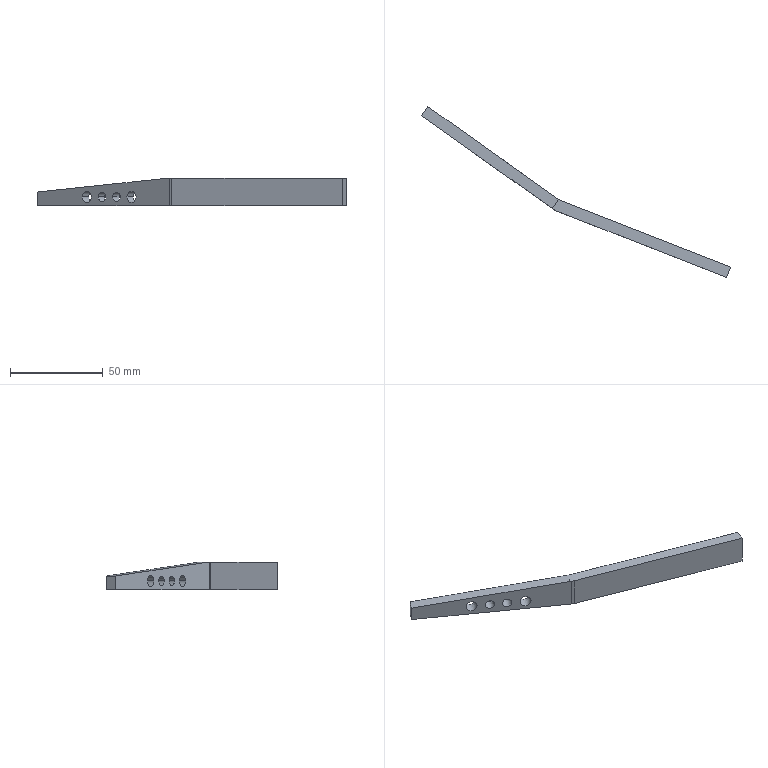Part | SolidWorks | features HoleWzd 2, Cut 1, Extrusion 1 | 1 solid | 19 faces | box 166.528 x 92.061 x 15 mm | volume 14282 mm3 | cylinder 10 | plane 9 | commonest cylinder face diameters 5 x4 6 x4 12 x2
STEP:
#1=CARTESIAN_POINT('',(-108.721,171.607,4.871));
#2=VERTEX_POINT('',#1);
#3=CARTESIAN_POINT('',(-112.797,174.503,4.871));
#4=VERTEX_POINT('',#3);
#5=CARTESIAN_POINT('',(-110.759,173.055,4.871));
#6=DIRECTION('',(0.5792,0.8152,0.));
#7=DIRECTION('',(-0.8152,0.5792,0.));
#8=AXIS2_PLACEMENT_3D('',#5,#6,#7);
#9=CIRCLE('',#8,2.5);
#10=EDGE_CURVE('',#2,#4,#9,.T.);
#11=ORIENTED_EDGE('',*,*,#10,.F.);
#12=CARTESIAN_POINT('',(-105.245,176.498,4.871));
#13=VERTEX_POINT('',#12);
#14=CARTESIAN_POINT('',(-105.245,176.498,4.871));
#15=DIRECTION('',(0.5792,0.8152,0.));
#16=VECTOR('',#15,1000.);
#17=LINE('',#14,#16);
#18=EDGE_CURVE('',#2,#13,#17,.T.);
#19=ORIENTED_EDGE('',*,*,#18,.T.);
#20=CARTESIAN_POINT('',(-109.321,179.394,4.871));
#21=VERTEX_POINT('',#20);
#22=CARTESIAN_POINT('',(-107.283,177.946,4.871));
#23=DIRECTION('',(0.5792,0.8152,0.));
#24=DIRECTION('',(-0.8152,0.5792,0.));
#25=AXIS2_PLACEMENT_3D('',#22,#23,#24);
#26=CIRCLE('',#25,2.5);
#27=EDGE_CURVE('',#13,#21,#26,.T.);
#28=ORIENTED_EDGE('',*,*,#27,.T.);
#29=CARTESIAN_POINT('',(-109.321,179.394,4.871));
#30=DIRECTION('',(0.5792,0.8152,0.));
#31=VECTOR('',#30,1000.);
#32=LINE('',#29,#31);
#33=EDGE_CURVE('',#4,#21,#32,.T.);
#34=ORIENTED_EDGE('',*,*,#33,.F.);
#35=EDGE_LOOP('',(#11,#19,#28,#34));
#36=FACE_OUTER_BOUND('',#35,.T.);
#37=CARTESIAN_POINT('',(-107.283,177.946,4.871));
#38=DIRECTION('',(0.5792,0.8152,0.));
#39=DIRECTION('',(-0.8152,0.5792,0.));
#40=AXIS2_PLACEMENT_3D('',#37,#38,#39);
#41=CYLINDRICAL_SURFACE('',#40,2.5);
#42=ADVANCED_FACE('',(#36),#41,.F.);
#43=CARTESIAN_POINT('',(-100.99,166.114,4.871));
#44=VERTEX_POINT('',#43);
#45=CARTESIAN_POINT('',(-105.066,169.01,4.871));
#46=VERTEX_POINT('',#45);
#47=CARTESIAN_POINT('',(-103.028,167.562,4.871));
#48=DIRECTION('',(0.5792,0.8152,0.));
#49=DIRECTION('',(-0.8152,0.5792,0.));
#50=AXIS2_PLACEMENT_3D('',#47,#48,#49);
#51=CIRCLE('',#50,2.5);
#52=EDGE_CURVE('',#44,#46,#51,.T.);
#53=ORIENTED_EDGE('',*,*,#52,.F.);
#54=CARTESIAN_POINT('',(-97.515,171.005,4.871));
#55=VERTEX_POINT('',#54);
#56=CARTESIAN_POINT('',(-97.515,171.005,4.871));
#57=DIRECTION('',(0.5792,0.8152,0.));
#58=VECTOR('',#57,1000.);
#59=LINE('',#56,#58);
#60=EDGE_CURVE('',#44,#55,#59,.T.);
#61=ORIENTED_EDGE('',*,*,#60,.T.);
#62=CARTESIAN_POINT('',(-101.591,173.901,4.871));
#63=VERTEX_POINT('',#62);
#64=CARTESIAN_POINT('',(-99.553,172.453,4.871));
#65=DIRECTION('',(0.5792,0.8152,0.));
#66=DIRECTION('',(-0.8152,0.5792,0.));
#67=AXIS2_PLACEMENT_3D('',#64,#65,#66);
#68=CIRCLE('',#67,2.5);
#69=EDGE_CURVE('',#55,#63,#68,.T.);
#70=ORIENTED_EDGE('',*,*,#69,.T.);
#71=CARTESIAN_POINT('',(-101.591,173.901,4.871));
#72=DIRECTION('',(0.5792,0.8152,0.));
#73=VECTOR('',#72,1000.);
#74=LINE('',#71,#73);
#75=EDGE_CURVE('',#46,#63,#74,.T.);
#76=ORIENTED_EDGE('',*,*,#75,.F.);
#77=EDGE_LOOP('',(#53,#61,#70,#76));
#78=FACE_OUTER_BOUND('',#77,.T.);
#79=CARTESIAN_POINT('',(-99.553,172.453,4.871));
#80=DIRECTION('',(0.5792,0.8152,0.));
#81=DIRECTION('',(-0.8152,0.5792,0.));
#82=AXIS2_PLACEMENT_3D('',#79,#80,#81);
#83=CYLINDRICAL_SURFACE('',#82,2.5);
#84=ADVANCED_FACE('',(#78),#83,.F.);
#85=CARTESIAN_POINT('',(-116.465,177.109,4.871));
#86=VERTEX_POINT('',#85);
#87=CARTESIAN_POINT('',(-121.356,180.584,4.871));
#88=VERTEX_POINT('',#87);
#89=CARTESIAN_POINT('',(-118.91,178.847,4.871));
#90=DIRECTION('',(0.5792,0.8152,0.));
#91=DIRECTION('',(-0.8152,0.5792,0.));
#92=AXIS2_PLACEMENT_3D('',#89,#90,#91);
#93=CIRCLE('',#92,3.);
#94=EDGE_CURVE('',#86,#88,#93,.T.);
#95=ORIENTED_EDGE('',*,*,#94,.F.);
#96=CARTESIAN_POINT('',(-112.99,182.,4.871));
#97=VERTEX_POINT('',#96);
#98=CARTESIAN_POINT('',(-112.99,182.,4.871));
#99=DIRECTION('',(0.5792,0.8152,0.));
#100=VECTOR('',#99,1000.);
#101=LINE('',#98,#100);
#102=EDGE_CURVE('',#86,#97,#101,.T.);
#103=ORIENTED_EDGE('',*,*,#102,.T.);
#104=CARTESIAN_POINT('',(-117.881,185.475,4.871));
#105=VERTEX_POINT('',#104);
#106=CARTESIAN_POINT('',(-115.435,183.738,4.871));
#107=DIRECTION('',(0.5792,0.8152,0.));
#108=DIRECTION('',(-0.8152,0.5792,0.));
#109=AXIS2_PLACEMENT_3D('',#106,#107,#108);
#110=CIRCLE('',#109,3.);
#111=EDGE_CURVE('',#97,#105,#110,.T.);
#112=ORIENTED_EDGE('',*,*,#111,.T.);
#113=CARTESIAN_POINT('',(-117.881,185.475,4.871));
#114=DIRECTION('',(0.5792,0.8152,0.));
#115=VECTOR('',#114,1000.);
#116=LINE('',#113,#115);
#117=EDGE_CURVE('',#88,#105,#116,.T.);
#118=ORIENTED_EDGE('',*,*,#117,.F.);
#119=EDGE_LOOP('',(#95,#103,#112,#118));
#120=FACE_OUTER_BOUND('',#119,.T.);
#121=CARTESIAN_POINT('',(-115.435,183.738,4.871));
#122=DIRECTION('',(0.5792,0.8152,0.));
#123=DIRECTION('',(-0.8152,0.5792,0.));
#124=AXIS2_PLACEMENT_3D('',#121,#122,#123);
#125=CYLINDRICAL_SURFACE('',#124,3.);
#126=ADVANCED_FACE('',(#120),#125,.F.);
#127=CARTESIAN_POINT('',(-92.431,160.032,4.871));
#128=VERTEX_POINT('',#127);
#129=CARTESIAN_POINT('',(-97.322,163.507,4.871));
#130=VERTEX_POINT('',#129);
#131=CARTESIAN_POINT('',(-94.876,161.77,4.871));
#132=DIRECTION('',(0.5792,0.8152,0.));
#133=DIRECTION('',(-0.8152,0.5792,0.));
#134=AXIS2_PLACEMENT_3D('',#131,#132,#133);
#135=CIRCLE('',#134,3.);
#136=EDGE_CURVE('',#128,#130,#135,.T.);
#137=ORIENTED_EDGE('',*,*,#136,.F.);
#138=CARTESIAN_POINT('',(-88.955,164.923,4.871));
#139=VERTEX_POINT('',#138);
#140=CARTESIAN_POINT('',(-88.955,164.923,4.871));
#141=DIRECTION('',(0.5792,0.8152,0.));
#142=VECTOR('',#141,1000.);
#143=LINE('',#140,#142);
#144=EDGE_CURVE('',#128,#139,#143,.T.);
#145=ORIENTED_EDGE('',*,*,#144,.T.);
#146=CARTESIAN_POINT('',(-93.846,168.398,4.871));
#147=VERTEX_POINT('',#146);
#148=CARTESIAN_POINT('',(-91.401,166.661,4.871));
#149=DIRECTION('',(0.5792,0.8152,0.));
#150=DIRECTION('',(-0.8152,0.5792,0.));
#151=AXIS2_PLACEMENT_3D('',#148,#149,#150);
#152=CIRCLE('',#151,3.);
#153=EDGE_CURVE('',#139,#147,#152,.T.);
#154=ORIENTED_EDGE('',*,*,#153,.T.);
#155=CARTESIAN_POINT('',(-93.846,168.398,4.871));
#156=DIRECTION('',(0.5792,0.8152,0.));
#157=VECTOR('',#156,1000.);
#158=LINE('',#155,#157);
#159=EDGE_CURVE('',#130,#147,#158,.T.);
#160=ORIENTED_EDGE('',*,*,#159,.F.);
#161=EDGE_LOOP('',(#137,#145,#154,#160));
#162=FACE_OUTER_BOUND('',#161,.T.);
#163=CARTESIAN_POINT('',(-91.401,166.661,4.871));
#164=DIRECTION('',(0.5792,0.8152,0.));
#165=DIRECTION('',(-0.8152,0.5792,0.));
#166=AXIS2_PLACEMENT_3D('',#163,#164,#165);
#167=CYLINDRICAL_SURFACE('',#166,3.);
#168=ADVANCED_FACE('',(#162),#167,.F.);
#169=CARTESIAN_POINT('',(-74.469,147.269,0.));
#170=VERTEX_POINT('',#169);
#171=CARTESIAN_POINT('',(-73.179,146.573,0.));
#172=VERTEX_POINT('',#171);
#173=CARTESIAN_POINT('',(-70.994,152.16,0.));
#174=DIRECTION('',(0.,0.,1.));
#175=DIRECTION('',(-1.,0.,0.));
#176=AXIS2_PLACEMENT_3D('',#173,#174,#175);
#177=CIRCLE('',#176,6.);
#178=EDGE_CURVE('',#170,#172,#177,.T.);
#179=ORIENTED_EDGE('',*,*,#178,.T.);
#180=CARTESIAN_POINT('',(-73.179,146.573,15.));
#181=VERTEX_POINT('',#180);
#182=CARTESIAN_POINT('',(-73.179,146.573,15.));
#183=DIRECTION('',(0.,0.,-1.));
#184=VECTOR('',#183,1000.);
#185=LINE('',#182,#184);
#186=EDGE_CURVE('',#181,#172,#185,.T.);
#187=ORIENTED_EDGE('',*,*,#186,.F.);
#188=CARTESIAN_POINT('',(-74.469,147.269,15.));
#189=VERTEX_POINT('',#188);
#190=CARTESIAN_POINT('',(-70.994,152.16,15.));
#191=DIRECTION('',(0.,0.,1.));
#192=DIRECTION('',(-1.,0.,0.));
#193=AXIS2_PLACEMENT_3D('',#190,#191,#192);
#194=CIRCLE('',#193,6.);
#195=EDGE_CURVE('',#189,#181,#194,.T.);
#196=ORIENTED_EDGE('',*,*,#195,.F.);
#197=CARTESIAN_POINT('',(-74.469,147.269,15.));
#198=DIRECTION('',(0.,0.,-1.));
#199=VECTOR('',#198,1000.);
#200=LINE('',#197,#199);
#201=EDGE_CURVE('',#189,#170,#200,.T.);
#202=ORIENTED_EDGE('',*,*,#201,.T.);
#203=EDGE_LOOP('',(#179,#187,#196,#202));
#204=FACE_OUTER_BOUND('',#203,.T.);
#205=CARTESIAN_POINT('',(-70.994,152.16,15.));
#206=DIRECTION('',(0.,0.,-1.));
#207=DIRECTION('',(-1.,0.,0.));
#208=AXIS2_PLACEMENT_3D('',#205,#206,#207);
#209=CYLINDRICAL_SURFACE('',#208,6.);
#210=ADVANCED_FACE('',(#204),#209,.T.);
#211=CARTESIAN_POINT('',(18.795,110.604,0.));
#212=VERTEX_POINT('',#211);
#213=CARTESIAN_POINT('',(-73.179,146.573,0.));
#214=DIRECTION('',(0.9313,-0.3642,0.));
#215=VECTOR('',#214,1000.);
#216=LINE('',#213,#215);
#217=EDGE_CURVE('',#172,#212,#216,.T.);
#218=ORIENTED_EDGE('',*,*,#217,.T.);
#219=CARTESIAN_POINT('',(18.795,110.604,15.));
#220=VERTEX_POINT('',#219);
#221=CARTESIAN_POINT('',(18.795,110.604,15.));
#222=DIRECTION('',(0.,0.,-1.));
#223=VECTOR('',#222,1000.);
#224=LINE('',#221,#223);
#225=EDGE_CURVE('',#220,#212,#224,.T.);
#226=ORIENTED_EDGE('',*,*,#225,.F.);
#227=CARTESIAN_POINT('',(-73.179,146.573,15.));
#228=DIRECTION('',(0.9313,-0.3642,0.));
#229=VECTOR('',#228,1000.);
#230=LINE('',#227,#229);
#231=EDGE_CURVE('',#181,#220,#230,.T.);
#232=ORIENTED_EDGE('',*,*,#231,.F.);
#233=ORIENTED_EDGE('',*,*,#186,.T.);
#234=EDGE_LOOP('',(#218,#226,#232,#233));
#235=FACE_OUTER_BOUND('',#234,.T.);
#236=CARTESIAN_POINT('',(-73.179,146.573,15.));
#237=DIRECTION('',(0.3642,0.9313,0.));
#238=DIRECTION('',(-0.9313,0.3642,0.));
#239=AXIS2_PLACEMENT_3D('',#236,#237,#238);
#240=PLANE('',#239);
#241=ADVANCED_FACE('',(#235),#240,.F.);
#242=CARTESIAN_POINT('',(20.981,116.192,0.));
#243=VERTEX_POINT('',#242);
#244=CARTESIAN_POINT('',(18.795,110.604,0.));
#245=DIRECTION('',(0.3642,0.9313,0.));
#246=VECTOR('',#245,1000.);
#247=LINE('',#244,#246);
#248=EDGE_CURVE('',#212,#243,#247,.T.);
#249=ORIENTED_EDGE('',*,*,#248,.T.);
#250=CARTESIAN_POINT('',(20.981,116.192,15.));
#251=VERTEX_POINT('',#250);
#252=CARTESIAN_POINT('',(20.981,116.192,15.));
#253=DIRECTION('',(0.,0.,-1.));
#254=VECTOR('',#253,1000.);
#255=LINE('',#252,#254);
#256=EDGE_CURVE('',#251,#243,#255,.T.);
#257=ORIENTED_EDGE('',*,*,#256,.F.);
#258=CARTESIAN_POINT('',(18.795,110.604,15.));
#259=DIRECTION('',(0.3642,0.9313,0.));
#260=VECTOR('',#259,1000.);
#261=LINE('',#258,#260);
#262=EDGE_CURVE('',#220,#251,#261,.T.);
#263=ORIENTED_EDGE('',*,*,#262,.F.);
#264=ORIENTED_EDGE('',*,*,#225,.T.);
#265=EDGE_LOOP('',(#249,#257,#263,#264));
#266=FACE_OUTER_BOUND('',#265,.T.);
#267=CARTESIAN_POINT('',(18.795,110.604,15.));
#268=DIRECTION('',(-0.9313,0.3642,0.));
#269=DIRECTION('',(-0.3642,-0.9313,0.));
#270=AXIS2_PLACEMENT_3D('',#267,#268,#269);
#271=PLANE('',#270);
#272=ADVANCED_FACE('',(#266),#271,.F.);
#273=CARTESIAN_POINT('',(-70.306,151.891,0.));
#274=VERTEX_POINT('',#273);
#275=CARTESIAN_POINT('',(-70.306,151.891,0.));
#276=DIRECTION('',(-0.9313,0.3642,0.));
#277=VECTOR('',#276,1000.);
#278=LINE('',#275,#277);
#279=EDGE_CURVE('',#243,#274,#278,.T.);
#280=ORIENTED_EDGE('',*,*,#279,.T.);
#281=CARTESIAN_POINT('',(-70.306,151.891,15.));
#282=VERTEX_POINT('',#281);
#283=CARTESIAN_POINT('',(-70.306,151.891,15.));
#284=DIRECTION('',(0.,0.,-1.));
#285=VECTOR('',#284,1000.);
#286=LINE('',#283,#285);
#287=EDGE_CURVE('',#282,#274,#286,.T.);
#288=ORIENTED_EDGE('',*,*,#287,.F.);
#289=CARTESIAN_POINT('',(-70.306,151.891,15.));
#290=DIRECTION('',(-0.9313,0.3642,0.));
#291=VECTOR('',#290,1000.);
#292=LINE('',#289,#291);
#293=EDGE_CURVE('',#251,#282,#292,.T.);
#294=ORIENTED_EDGE('',*,*,#293,.F.);
#295=ORIENTED_EDGE('',*,*,#256,.T.);
#296=EDGE_LOOP('',(#280,#288,#294,#295));
#297=FACE_OUTER_BOUND('',#296,.T.);
#298=CARTESIAN_POINT('',(-70.306,151.891,15.));
#299=DIRECTION('',(-0.3642,-0.9313,0.));
#300=DIRECTION('',(0.9313,-0.3642,0.));
#301=AXIS2_PLACEMENT_3D('',#298,#299,#300);
#302=PLANE('',#301);
#303=ADVANCED_FACE('',(#297),#302,.F.);
#304=CARTESIAN_POINT('',(-71.596,152.588,0.));
#305=VERTEX_POINT('',#304);
#306=CARTESIAN_POINT('',(-68.121,157.479,0.));
#307=DIRECTION('',(0.,0.,-1.));
#308=DIRECTION('',(-1.,0.,0.));
#309=AXIS2_PLACEMENT_3D('',#306,#307,#308);
#310=CIRCLE('',#309,6.);
#311=EDGE_CURVE('',#274,#305,#310,.T.);
#312=ORIENTED_EDGE('',*,*,#311,.T.);
#313=CARTESIAN_POINT('',(-71.596,152.588,15.));
#314=VERTEX_POINT('',#313);
#315=CARTESIAN_POINT('',(-71.596,152.588,15.));
#316=DIRECTION('',(0.,0.,-1.));
#317=VECTOR('',#316,1000.);
#318=LINE('',#315,#317);
#319=EDGE_CURVE('',#314,#305,#318,.T.);
#320=ORIENTED_EDGE('',*,*,#319,.F.);
#321=CARTESIAN_POINT('',(-68.121,157.479,15.));
#322=DIRECTION('',(0.,0.,-1.));
#323=DIRECTION('',(-1.,0.,0.));
#324=AXIS2_PLACEMENT_3D('',#321,#322,#323);
#325=CIRCLE('',#324,6.);
#326=EDGE_CURVE('',#282,#314,#325,.T.);
#327=ORIENTED_EDGE('',*,*,#326,.F.);
#328=ORIENTED_EDGE('',*,*,#287,.T.);
#329=EDGE_LOOP('',(#312,#320,#327,#328));
#330=FACE_OUTER_BOUND('',#329,.T.);
#331=CARTESIAN_POINT('',(-68.121,157.479,15.));
#332=DIRECTION('',(0.,0.,-1.));
#333=DIRECTION('',(-1.,0.,0.));
#334=AXIS2_PLACEMENT_3D('',#331,#332,#333);
#335=CYLINDRICAL_SURFACE('',#334,6.);
#336=ADVANCED_FACE('',(#330),#335,.F.);
#337=CARTESIAN_POINT('',(-107.283,177.946,4.871));
#338=DIRECTION('',(0.5792,0.8152,0.));
#339=DIRECTION('',(-0.8152,0.5792,0.));
#340=AXIS2_PLACEMENT_3D('',#337,#338,#339);
#341=CIRCLE('',#340,2.5);
#342=EDGE_CURVE('',#21,#13,#341,.T.);
#343=ORIENTED_EDGE('',*,*,#342,.F.);
#344=ORIENTED_EDGE('',*,*,#27,.F.);
#345=EDGE_LOOP('',(#343,#344));
#346=FACE_BOUND('',#345,.T.);
#347=CARTESIAN_POINT('',(-99.553,172.453,4.871));
#348=DIRECTION('',(0.5792,0.8152,0.));
#349=DIRECTION('',(-0.8152,0.5792,0.));
#350=AXIS2_PLACEMENT_3D('',#347,#348,#349);
#351=CIRCLE('',#350,2.5);
#352=EDGE_CURVE('',#63,#55,#351,.T.);
#353=ORIENTED_EDGE('',*,*,#352,.F.);
#354=ORIENTED_EDGE('',*,*,#69,.F.);
#355=EDGE_LOOP('',(#353,#354));
#356=FACE_BOUND('',#355,.T.);
#357=CARTESIAN_POINT('',(-115.435,183.738,4.871));
#358=DIRECTION('',(0.5792,0.8152,0.));
#359=DIRECTION('',(-0.8152,0.5792,0.));
#360=AXIS2_PLACEMENT_3D('',#357,#358,#359);
#361=CIRCLE('',#360,3.);
#362=EDGE_CURVE('',#105,#97,#361,.T.);
#363=ORIENTED_EDGE('',*,*,#362,.F.);
#364=ORIENTED_EDGE('',*,*,#111,.F.);
#365=EDGE_LOOP('',(#363,#364));
#366=FACE_BOUND('',#365,.T.);
#367=CARTESIAN_POINT('',(-91.401,166.661,4.871));
#368=DIRECTION('',(0.5792,0.8152,0.));
#369=DIRECTION('',(-0.8152,0.5792,0.));
#370=AXIS2_PLACEMENT_3D('',#367,#368,#369);
#371=CIRCLE('',#370,3.);
#372=EDGE_CURVE('',#147,#139,#371,.T.);
#373=ORIENTED_EDGE('',*,*,#372,.F.);
#374=ORIENTED_EDGE('',*,*,#153,.F.);
#375=EDGE_LOOP('',(#373,#374));
#376=FACE_BOUND('',#375,.T.);
#377=CARTESIAN_POINT('',(-142.072,202.665,7.5));
#378=VERTEX_POINT('',#377);
#379=CARTESIAN_POINT('',(-142.072,202.665,0.));
#380=VERTEX_POINT('',#379);
#381=CARTESIAN_POINT('',(-142.072,202.665,15.));
#382=DIRECTION('',(0.,0.,-1.));
#383=VECTOR('',#382,1000.);
#384=LINE('',#381,#383);
#385=EDGE_CURVE('',#378,#380,#384,.T.);
#386=ORIENTED_EDGE('',*,*,#385,.F.);
#387=CARTESIAN_POINT('',(-142.072,202.665,7.5));
#388=DIRECTION('',(-0.8121,0.577,-0.08643));
#389=VECTOR('',#388,1000.);
#390=LINE('',#387,#389);
#391=EDGE_CURVE('',#314,#378,#390,.T.);
#392=ORIENTED_EDGE('',*,*,#391,.F.);
#393=ORIENTED_EDGE('',*,*,#319,.T.);
#394=CARTESIAN_POINT('',(-142.072,202.665,0.));
#395=DIRECTION('',(-0.8152,0.5792,0.));
#396=VECTOR('',#395,1000.);
#397=LINE('',#394,#396);
#398=EDGE_CURVE('',#305,#380,#397,.T.);
#399=ORIENTED_EDGE('',*,*,#398,.T.);
#400=EDGE_LOOP('',(#386,#392,#393,#399));
#401=FACE_OUTER_BOUND('',#400,.T.);
#402=CARTESIAN_POINT('',(-142.072,202.665,15.));
#403=DIRECTION('',(-0.5792,-0.8152,0.));
#404=DIRECTION('',(0.8152,-0.5792,0.));
#405=AXIS2_PLACEMENT_3D('',#402,#403,#404);
#406=PLANE('',#405);
#407=ADVANCED_FACE('',(#346,#356,#366,#376,#401),#406,.F.);
#408=CARTESIAN_POINT('',(-145.547,197.774,7.5));
#409=VERTEX_POINT('',#408);
#410=CARTESIAN_POINT('',(-145.547,197.774,0.));
#411=VERTEX_POINT('',#410);
#412=CARTESIAN_POINT('',(-145.547,197.774,15.));
#413=DIRECTION('',(0.,0.,-1.));
#414=VECTOR('',#413,1000.);
#415=LINE('',#412,#414);
#416=EDGE_CURVE('',#409,#411,#415,.T.);
#417=ORIENTED_EDGE('',*,*,#416,.F.);
#418=CARTESIAN_POINT('',(-153.656,186.361,7.5));
#419=DIRECTION('',(0.5792,0.8152,0.));
#420=VECTOR('',#419,1000.);
#421=LINE('',#418,#420);
#422=EDGE_CURVE('',#409,#378,#421,.T.);
#423=ORIENTED_EDGE('',*,*,#422,.T.);
#424=ORIENTED_EDGE('',*,*,#385,.T.);
#425=CARTESIAN_POINT('',(-145.547,197.774,0.));
#426=DIRECTION('',(-0.5792,-0.8152,0.));
#427=VECTOR('',#426,1000.);
#428=LINE('',#425,#427);
#429=EDGE_CURVE('',#380,#411,#428,.T.);
#430=ORIENTED_EDGE('',*,*,#429,.T.);
#431=EDGE_LOOP('',(#417,#423,#424,#430));
#432=FACE_OUTER_BOUND('',#431,.T.);
#433=CARTESIAN_POINT('',(-145.547,197.774,15.));
#434=DIRECTION('',(0.8152,-0.5792,0.));
#435=DIRECTION('',(0.5792,0.8152,0.));
#436=AXIS2_PLACEMENT_3D('',#433,#434,#435);
#437=PLANE('',#436);
#438=ADVANCED_FACE('',(#432),#437,.F.);
#439=CARTESIAN_POINT('',(-110.759,173.055,4.871));
#440=DIRECTION('',(0.5792,0.8152,0.));
#441=DIRECTION('',(-0.8152,0.5792,0.));
#442=AXIS2_PLACEMENT_3D('',#439,#440,#441);
#443=CIRCLE('',#442,2.5);
#444=EDGE_CURVE('',#4,#2,#443,.T.);
#445=ORIENTED_EDGE('',*,*,#444,.T.);
#446=ORIENTED_EDGE('',*,*,#10,.T.);
#447=EDGE_LOOP('',(#445,#446));
#448=FACE_BOUND('',#447,.T.);
#449=CARTESIAN_POINT('',(-103.028,167.562,4.871));
#450=DIRECTION('',(0.5792,0.8152,0.));
#451=DIRECTION('',(-0.8152,0.5792,0.));
#452=AXIS2_PLACEMENT_3D('',#449,#450,#451);
#453=CIRCLE('',#452,2.5);
#454=EDGE_CURVE('',#46,#44,#453,.T.);
#455=ORIENTED_EDGE('',*,*,#454,.T.);
#456=ORIENTED_EDGE('',*,*,#52,.T.);
#457=EDGE_LOOP('',(#455,#456));
#458=FACE_BOUND('',#457,.T.);
#459=CARTESIAN_POINT('',(-118.91,178.847,4.871));
#460=DIRECTION('',(0.5792,0.8152,0.));
#461=DIRECTION('',(-0.8152,0.5792,0.));
#462=AXIS2_PLACEMENT_3D('',#459,#460,#461);
#463=CIRCLE('',#462,3.);
#464=EDGE_CURVE('',#88,#86,#463,.T.);
#465=ORIENTED_EDGE('',*,*,#464,.T.);
#466=ORIENTED_EDGE('',*,*,#94,.T.);
#467=EDGE_LOOP('',(#465,#466));
#468=FACE_BOUND('',#467,.T.);
#469=CARTESIAN_POINT('',(-94.876,161.77,4.871));
#470=DIRECTION('',(0.5792,0.8152,0.));
#471=DIRECTION('',(-0.8152,0.5792,0.));
#472=AXIS2_PLACEMENT_3D('',#469,#470,#471);
#473=CIRCLE('',#472,3.);
#474=EDGE_CURVE('',#130,#128,#473,.T.);
#475=ORIENTED_EDGE('',*,*,#474,.T.);
#476=ORIENTED_EDGE('',*,*,#136,.T.);
#477=EDGE_LOOP('',(#475,#476));
#478=FACE_BOUND('',#477,.T.);
#479=CARTESIAN_POINT('',(-75.071,147.697,15.));
#480=VERTEX_POINT('',#479);
#481=CARTESIAN_POINT('',(-145.547,197.774,15.));
#482=DIRECTION('',(0.8152,-0.5792,0.));
#483=VECTOR('',#482,1000.);
#484=LINE('',#481,#483);
#485=EDGE_CURVE('',#480,#189,#484,.T.);
#486=ORIENTED_EDGE('',*,*,#485,.F.);
#487=CARTESIAN_POINT('',(-145.021,197.4,7.556));
#488=DIRECTION('',(-0.8121,0.577,-0.08643));
#489=VECTOR('',#488,1000.);
#490=LINE('',#487,#489);
#491=EDGE_CURVE('',#480,#409,#490,.T.);
#492=ORIENTED_EDGE('',*,*,#491,.T.);
#493=ORIENTED_EDGE('',*,*,#416,.T.);
#494=CARTESIAN_POINT('',(-145.547,197.774,0.));
#495=DIRECTION('',(0.8152,-0.5792,0.));
#496=VECTOR('',#495,1000.);
#497=LINE('',#494,#496);
#498=EDGE_CURVE('',#411,#170,#497,.T.);
#499=ORIENTED_EDGE('',*,*,#498,.T.);
#500=ORIENTED_EDGE('',*,*,#201,.F.);
#501=EDGE_LOOP('',(#486,#492,#493,#499,#500));
#502=FACE_OUTER_BOUND('',#501,.T.);
#503=CARTESIAN_POINT('',(-145.547,197.774,15.));
#504=DIRECTION('',(0.5792,0.8152,0.));
#505=DIRECTION('',(-0.8152,0.5792,0.));
#506=AXIS2_PLACEMENT_3D('',#503,#504,#505);
#507=PLANE('',#506);
#508=ADVANCED_FACE('',(#448,#458,#468,#478,#502),#507,.F.);
#509=ORIENTED_EDGE('',*,*,#326,.T.);
#510=CARTESIAN_POINT('',(-71.596,152.588,15.));
#511=DIRECTION('',(-0.5792,-0.8152,0.));
#512=VECTOR('',#511,1000.);
#513=LINE('',#510,#512);
#514=EDGE_CURVE('',#314,#480,#513,.T.);
#515=ORIENTED_EDGE('',*,*,#514,.T.);
#516=ORIENTED_EDGE('',*,*,#485,.T.);
#517=ORIENTED_EDGE('',*,*,#195,.T.);
#518=ORIENTED_EDGE('',*,*,#231,.T.);
#519=ORIENTED_EDGE('',*,*,#262,.T.);
#520=ORIENTED_EDGE('',*,*,#293,.T.);
#521=EDGE_LOOP('',(#509,#515,#516,#517,#518,#519,#520));
#522=FACE_OUTER_BOUND('',#521,.T.);
#523=CARTESIAN_POINT('',(-70.994,152.16,15.));
#524=DIRECTION('',(0.,0.,-1.));
#525=DIRECTION('',(-1.,0.,0.));
#526=AXIS2_PLACEMENT_3D('',#523,#524,#525);
#527=PLANE('',#526);
#528=ADVANCED_FACE('',(#522),#527,.F.);
#529=ORIENTED_EDGE('',*,*,#178,.F.);
#530=ORIENTED_EDGE('',*,*,#498,.F.);
#531=ORIENTED_EDGE('',*,*,#429,.F.);
#532=ORIENTED_EDGE('',*,*,#398,.F.);
#533=ORIENTED_EDGE('',*,*,#311,.F.);
#534=ORIENTED_EDGE('',*,*,#279,.F.);
#535=ORIENTED_EDGE('',*,*,#248,.F.);
#536=ORIENTED_EDGE('',*,*,#217,.F.);
#537=EDGE_LOOP('',(#529,#530,#531,#532,#533,#534,#535,#536));
#538=FACE_OUTER_BOUND('',#537,.T.);
#539=CARTESIAN_POINT('',(-70.994,152.16,0.));
#540=DIRECTION('',(0.,0.,-1.));
#541=DIRECTION('',(-1.,0.,0.));
#542=AXIS2_PLACEMENT_3D('',#539,#540,#541);
#543=PLANE('',#542);
#544=ADVANCED_FACE('',(#538),#543,.T.);
#545=ORIENTED_EDGE('',*,*,#514,.F.);
#546=ORIENTED_EDGE('',*,*,#391,.T.);
#547=ORIENTED_EDGE('',*,*,#422,.F.);
#548=ORIENTED_EDGE('',*,*,#491,.F.);
#549=EDGE_LOOP('',(#545,#546,#547,#548));
#550=FACE_OUTER_BOUND('',#549,.T.);
#551=CARTESIAN_POINT('',(-153.656,186.361,7.5));
#552=DIRECTION('',(0.07045,-0.05006,-0.9963));
#553=DIRECTION('',(-0.9975,0.,-0.07054));
#554=AXIS2_PLACEMENT_3D('',#551,#552,#553);
#555=PLANE('',#554);
#556=ADVANCED_FACE('',(#550),#555,.F.);
#557=ORIENTED_EDGE('',*,*,#144,.F.);
#558=ORIENTED_EDGE('',*,*,#474,.F.);
#559=ORIENTED_EDGE('',*,*,#159,.T.);
#560=ORIENTED_EDGE('',*,*,#372,.T.);
#561=EDGE_LOOP('',(#557,#558,#559,#560));
#562=FACE_OUTER_BOUND('',#561,.T.);
#563=CARTESIAN_POINT('',(-91.401,166.661,4.871));
#564=DIRECTION('',(0.5792,0.8152,0.));
#565=DIRECTION('',(-0.8152,0.5792,0.));
#566=AXIS2_PLACEMENT_3D('',#563,#564,#565);
#567=CYLINDRICAL_SURFACE('',#566,3.);
#568=ADVANCED_FACE('',(#562),#567,.F.);
#569=ORIENTED_EDGE('',*,*,#102,.F.);
#570=ORIENTED_EDGE('',*,*,#464,.F.);
#571=ORIENTED_EDGE('',*,*,#117,.T.);
#572=ORIENTED_EDGE('',*,*,#362,.T.);
#573=EDGE_LOOP('',(#569,#570,#571,#572));
#574=FACE_OUTER_BOUND('',#573,.T.);
#575=CARTESIAN_POINT('',(-115.435,183.738,4.871));
#576=DIRECTION('',(0.5792,0.8152,0.));
#577=DIRECTION('',(-0.8152,0.5792,0.));
#578=AXIS2_PLACEMENT_3D('',#575,#576,#577);
#579=CYLINDRICAL_SURFACE('',#578,3.);
#580=ADVANCED_FACE('',(#574),#579,.F.);
#581=ORIENTED_EDGE('',*,*,#60,.F.);
#582=ORIENTED_EDGE('',*,*,#454,.F.);
#583=ORIENTED_EDGE('',*,*,#75,.T.);
#584=ORIENTED_EDGE('',*,*,#352,.T.);
#585=EDGE_LOOP('',(#581,#582,#583,#584));
#586=FACE_OUTER_BOUND('',#585,.T.);
#587=CARTESIAN_POINT('',(-99.553,172.453,4.871));
#588=DIRECTION('',(0.5792,0.8152,0.));
#589=DIRECTION('',(-0.8152,0.5792,0.));
#590=AXIS2_PLACEMENT_3D('',#587,#588,#589);
#591=CYLINDRICAL_SURFACE('',#590,2.5);
#592=ADVANCED_FACE('',(#586),#591,.F.);
#593=ORIENTED_EDGE('',*,*,#18,.F.);
#594=ORIENTED_EDGE('',*,*,#444,.F.);
#595=ORIENTED_EDGE('',*,*,#33,.T.);
#596=ORIENTED_EDGE('',*,*,#342,.T.);
#597=EDGE_LOOP('',(#593,#594,#595,#596));
#598=FACE_OUTER_BOUND('',#597,.T.);
#599=CARTESIAN_POINT('',(-107.283,177.946,4.871));
#600=DIRECTION('',(0.5792,0.8152,0.));
#601=DIRECTION('',(-0.8152,0.5792,0.));
#602=AXIS2_PLACEMENT_3D('',#599,#600,#601);
#603=CYLINDRICAL_SURFACE('',#602,2.5);
#604=ADVANCED_FACE('',(#598),#603,.F.);
#605=CLOSED_SHELL('',(#42,#84,#126,#168,#210,#241,#272,#303,#336,#407,#438,#508,#528,#544,#556,#568,#580,#592,#604));
#606=MANIFOLD_SOLID_BREP('',#605);
#607=CARTESIAN_POINT('',(0.,0.,0.));
#608=DIRECTION('',(0.,0.,1.));
#609=DIRECTION('',(1.,0.,0.));
#610=AXIS2_PLACEMENT_3D('',#607,#608,#609);
#611=(LENGTH_UNIT()NAMED_UNIT(*)SI_UNIT(.MILLI.,.METRE.));
#612=UNCERTAINTY_MEASURE_WITH_UNIT(LENGTH_MEASURE(0.00001),#611,'','');
#613=(NAMED_UNIT(*)PLANE_ANGLE_UNIT()SI_UNIT($,.RADIAN.));
#614=(NAMED_UNIT(*)SI_UNIT($,.STERADIAN.)SOLID_ANGLE_UNIT());
#615=(GEOMETRIC_REPRESENTATION_CONTEXT(3)GLOBAL_UNCERTAINTY_ASSIGNED_CONTEXT((#612))GLOBAL_UNIT_ASSIGNED_CONTEXT((#611,#613,#614))REPRESENTATION_CONTEXT('',''));
#616=ADVANCED_BREP_SHAPE_REPRESENTATION('',(#606,#610),#615);